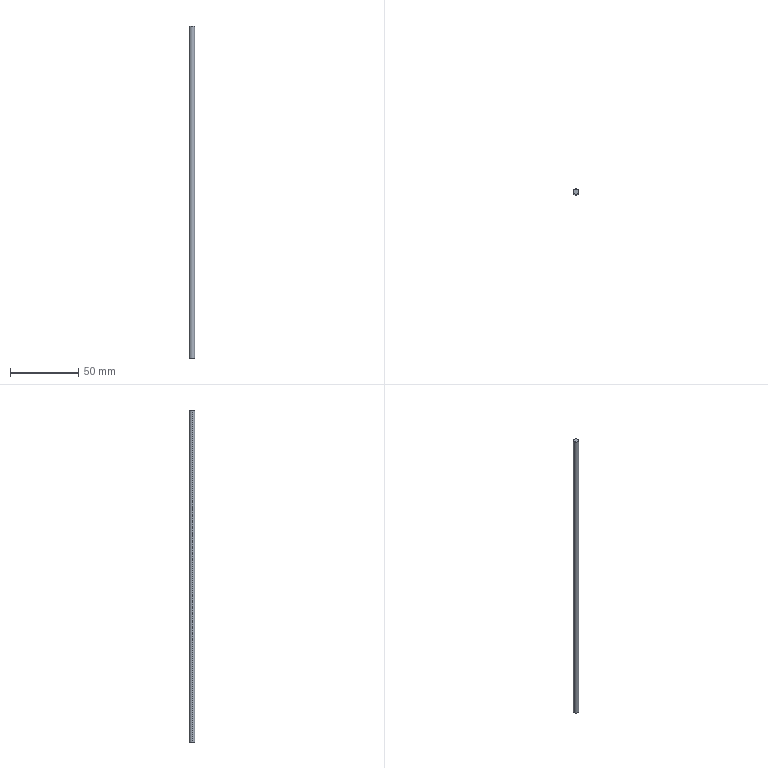Part | SolidWorks | features Extrusion 1 | 1 solid | 4 faces | box 4 x 4 x 242.5 mm | volume 3047 mm3 | cylinder 2 | plane 2 | commonest cylinder face diameters 4 x2
STEP:
#1=CARTESIAN_POINT('',(2.,0.,242.5));
#2=VERTEX_POINT('',#1);
#3=CARTESIAN_POINT('',(-2.,0.,242.5));
#4=VERTEX_POINT('',#3);
#5=CARTESIAN_POINT('',(0.,0.,242.5));
#6=DIRECTION('',(0.,0.,1.));
#7=DIRECTION('',(1.,0.,0.));
#8=AXIS2_PLACEMENT_3D('',#5,#6,#7);
#9=CIRCLE('',#8,2.);
#10=EDGE_CURVE('',#2,#4,#9,.T.);
#11=ORIENTED_EDGE('',*,*,#10,.F.);
#12=CARTESIAN_POINT('',(2.,0.,0.));
#13=VERTEX_POINT('',#12);
#14=CARTESIAN_POINT('',(2.,0.,242.5));
#15=DIRECTION('',(0.,0.,-1.));
#16=VECTOR('',#15,1000.);
#17=LINE('',#14,#16);
#18=EDGE_CURVE('',#2,#13,#17,.T.);
#19=ORIENTED_EDGE('',*,*,#18,.T.);
#20=CARTESIAN_POINT('',(-2.,0.,0.));
#21=VERTEX_POINT('',#20);
#22=CARTESIAN_POINT('',(0.,0.,0.));
#23=DIRECTION('',(0.,0.,1.));
#24=DIRECTION('',(1.,0.,0.));
#25=AXIS2_PLACEMENT_3D('',#22,#23,#24);
#26=CIRCLE('',#25,2.);
#27=EDGE_CURVE('',#13,#21,#26,.T.);
#28=ORIENTED_EDGE('',*,*,#27,.T.);
#29=CARTESIAN_POINT('',(-2.,0.,242.5));
#30=DIRECTION('',(0.,0.,-1.));
#31=VECTOR('',#30,1000.);
#32=LINE('',#29,#31);
#33=EDGE_CURVE('',#4,#21,#32,.T.);
#34=ORIENTED_EDGE('',*,*,#33,.F.);
#35=EDGE_LOOP('',(#11,#19,#28,#34));
#36=FACE_OUTER_BOUND('',#35,.T.);
#37=CARTESIAN_POINT('',(0.,0.,242.5));
#38=DIRECTION('',(0.,0.,-1.));
#39=DIRECTION('',(-1.,0.,0.));
#40=AXIS2_PLACEMENT_3D('',#37,#38,#39);
#41=CYLINDRICAL_SURFACE('',#40,2.);
#42=ADVANCED_FACE('',(#36),#41,.T.);
#43=ORIENTED_EDGE('',*,*,#18,.F.);
#44=CARTESIAN_POINT('',(0.,0.,242.5));
#45=DIRECTION('',(0.,0.,1.));
#46=DIRECTION('',(1.,0.,0.));
#47=AXIS2_PLACEMENT_3D('',#44,#45,#46);
#48=CIRCLE('',#47,2.);
#49=EDGE_CURVE('',#4,#2,#48,.T.);
#50=ORIENTED_EDGE('',*,*,#49,.F.);
#51=ORIENTED_EDGE('',*,*,#33,.T.);
#52=CARTESIAN_POINT('',(0.,0.,0.));
#53=DIRECTION('',(0.,0.,1.));
#54=DIRECTION('',(1.,0.,0.));
#55=AXIS2_PLACEMENT_3D('',#52,#53,#54);
#56=CIRCLE('',#55,2.);
#57=EDGE_CURVE('',#21,#13,#56,.T.);
#58=ORIENTED_EDGE('',*,*,#57,.T.);
#59=EDGE_LOOP('',(#43,#50,#51,#58));
#60=FACE_OUTER_BOUND('',#59,.T.);
#61=CARTESIAN_POINT('',(0.,0.,242.5));
#62=DIRECTION('',(0.,0.,-1.));
#63=DIRECTION('',(-1.,0.,0.));
#64=AXIS2_PLACEMENT_3D('',#61,#62,#63);
#65=CYLINDRICAL_SURFACE('',#64,2.);
#66=ADVANCED_FACE('',(#60),#65,.T.);
#67=ORIENTED_EDGE('',*,*,#49,.T.);
#68=ORIENTED_EDGE('',*,*,#10,.T.);
#69=EDGE_LOOP('',(#67,#68));
#70=FACE_OUTER_BOUND('',#69,.T.);
#71=CARTESIAN_POINT('',(0.,0.,242.5));
#72=DIRECTION('',(0.,0.,1.));
#73=DIRECTION('',(1.,0.,0.));
#74=AXIS2_PLACEMENT_3D('',#71,#72,#73);
#75=PLANE('',#74);
#76=ADVANCED_FACE('',(#70),#75,.T.);
#77=ORIENTED_EDGE('',*,*,#57,.F.);
#78=ORIENTED_EDGE('',*,*,#27,.F.);
#79=EDGE_LOOP('',(#77,#78));
#80=FACE_OUTER_BOUND('',#79,.T.);
#81=CARTESIAN_POINT('',(0.,0.,0.));
#82=DIRECTION('',(0.,0.,1.));
#83=DIRECTION('',(1.,0.,0.));
#84=AXIS2_PLACEMENT_3D('',#81,#82,#83);
#85=PLANE('',#84);
#86=ADVANCED_FACE('',(#80),#85,.F.);
#87=CLOSED_SHELL('',(#42,#66,#76,#86));
#88=MANIFOLD_SOLID_BREP('',#87);
#89=CARTESIAN_POINT('',(0.,0.,0.));
#90=DIRECTION('',(0.,0.,1.));
#91=DIRECTION('',(1.,0.,0.));
#92=AXIS2_PLACEMENT_3D('',#89,#90,#91);
#93=(LENGTH_UNIT()NAMED_UNIT(*)SI_UNIT(.MILLI.,.METRE.));
#94=UNCERTAINTY_MEASURE_WITH_UNIT(LENGTH_MEASURE(0.00001),#93,'','');
#95=(NAMED_UNIT(*)PLANE_ANGLE_UNIT()SI_UNIT($,.RADIAN.));
#96=(NAMED_UNIT(*)SI_UNIT($,.STERADIAN.)SOLID_ANGLE_UNIT());
#97=(GEOMETRIC_REPRESENTATION_CONTEXT(3)GLOBAL_UNCERTAINTY_ASSIGNED_CONTEXT((#94))GLOBAL_UNIT_ASSIGNED_CONTEXT((#93,#95,#96))REPRESENTATION_CONTEXT('',''));
#98=ADVANCED_BREP_SHAPE_REPRESENTATION('',(#88,#92),#97);